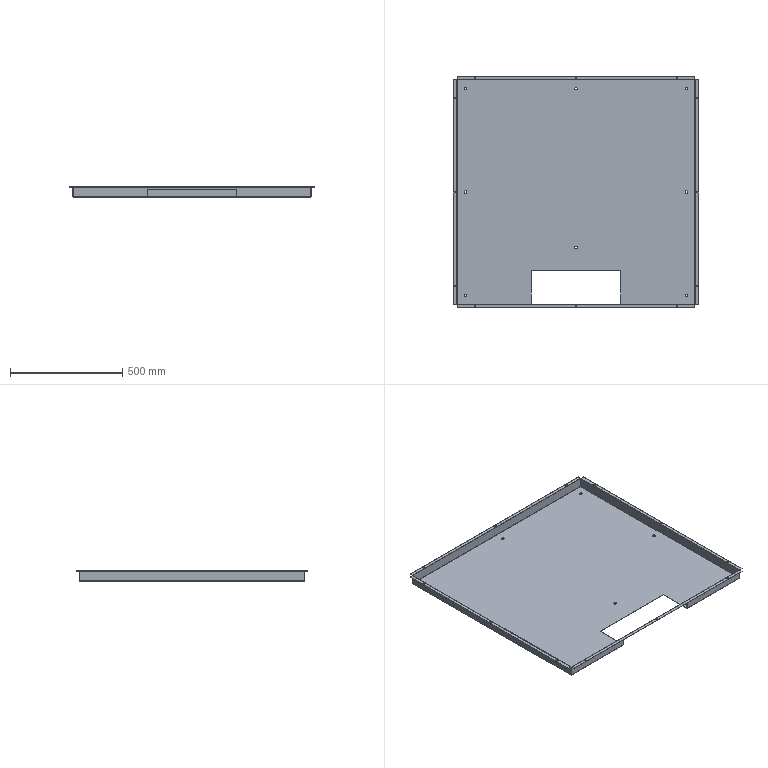Part | SolidWorks | features ICE 4, EdgeFlange 2, FlatPattern 1, SMBaseFlange 1, SheetMetal 1 | 1 solid | 150 faces | box 1095 x 1035 x 45 mm | volume 1236124 mm3 | plane 78 | cylinder 64 | spline 8 | commonest cylinder face diameters 7 x30 11 x16 0.4 x9 2.4 x9